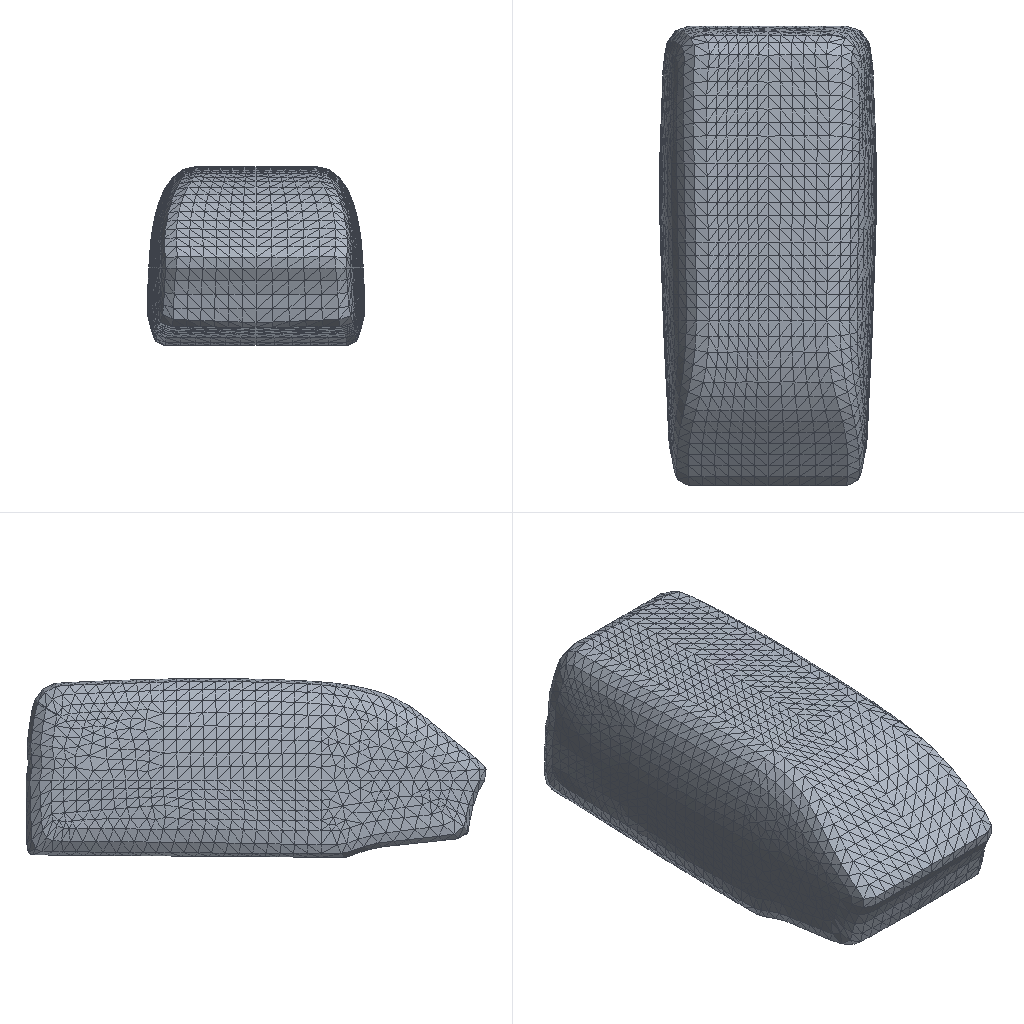Simulation study | abaqus
Set-up summary:
category,name,step,type,value,unit,region
solver,abaqus
solver,version,,,Abaqus/Standard 2020
units,not stated in the deck,,not stated
analysis,deck,,static,static
load_step,Step-1,Step-1,static
load_step,requested,,,1
mesh,nodes,,,7411
mesh,elements,,,37750
element_type,C3D4,,solid,37750
load,load commands in deck,,count,5
bc,support commands in deck,,count,2
material,MATERIAL-1,,in results
check,setup vs results,,match,"per instance, exact: element labels, types and connectivity; labels of the nodes the elements use; coordinates of those nodes at SINGLE_PRECISION in 1 of 1 instance(s)"
Abaqus input file, long lists of numbers shortened:
*Heading
** Job name: Job-3 Model name: Model-3
** Generated by: Abaqus/CAE 2020
*Preprint, echo=NO, model=NO, history=NO, contact=NO
**
** PARTS
**
*Part, name=car3
*Node
      1,   6696.368,        2333.,   520.596
      2,    6753.329,   1345.336,   -47.678
** (7409 more lines like these left out)
*Element, type=C3D4
    1, 2254, 2255, 2256, 2257
    2, 2254, 2256, 2258, 2259
** (37748 more lines like these left out)
*Nset, nset=Set-5, generate
    1,  7411,     1
*Elset, elset=Set-5, generate
     1,  37750,      1
** Section: Section-1
*Solid Section, elset=Set-5, material=Material-1
,
*End Part
**
**
** ASSEMBLY
**
*Assembly, name=Assembly
**
*Instance, name=car3-1, part=car3
*End Instance
**
*Node
      1,   6003.251,   1382.023,  -167.344
*Nset, nset=Set-1, instance=car3-1
    1,    2,    3,    4,    7,    9,   10,   11,   12,   13,   14,   17,   18,   19,   20,   22
   24,   25,   35,   37,   38,   40,   41,   47,   48,   51,   52,   55,   56,   57,   58,   60
** (41 more lines like these left out)
*Elset, elset=Set-1, instance=car3-1
   344,   416,   559,   823,  1168,  1393,  1583,  1620,  2065,  2093,  2105,  2139,  2392,  2495,  2498,  2530
  2554,  2560,  2567,  2572,  2579,  2583,  2603,  2620,  2644,  2647,  2648,  2671,  2673,  2676,  2677,  2683
** (68 more lines like these left out)
*Nset, nset=Set-4
 1,
*Nset, nset=m_Set-2
 1,
*Nset, nset=s_Set-2, instance=car3-1
   29,   30,   42,  283,  284,  285,  286,  287,  288,  289,  290,  291,  292,  293,  294,  295
  296,  297,  298,  299,  300,  301,  302,  303,  304,  382,  383,  384,  385,  386,  387,  388
** (6 more lines like these left out)
*Elset, elset=s_Set-2, instance=car3-1
  2316,  2317,  2608,  2732,  2791,  2832,  2979,  3086,  3128,  3158,  3826,  3863,  3878,  3887,  3889,  4278
  4320,  4345,  4360,  4364,  4367,  4375,  4383,  4407,  4409,  4415,  4429,  4472,  4497,  4509,  4541,  4543
** (12 more lines like these left out)
*Elset, elset=_Surf-1_S2, internal, instance=car3-1
   283,  3506,  3571,  3768,  4714,  5221,  5234,  5363,  5465,  7511, 19785, 23410, 25854
*Elset, elset=_Surf-1_S3, internal, instance=car3-1
   555,   614,  1939,  2150,  2281,  2592,  2668,  2698,  2714,  2740,  2771,  2981,  2997,  3073,  3129,  3131
  3161,  3234,  3238,  3257,  3269,  3308,  3318,  3321,  3339,  3341,  3361,  3368,  3369,  3370,  3378,  3398
** (10 more lines like these left out)
*Elset, elset=_Surf-1_S1, internal, instance=car3-1
  2723,  3423,  3520,  4402,  4690,  5366, 17848, 19788, 30557, 33192
*Elset, elset=_Surf-1_S4, internal, instance=car3-1
  3097,  4419,  4611,  5518,  9574, 15637, 22914, 28537
*Surface, type=ELEMENT, name=Surf-1
_Surf-1_S2, S2
_Surf-1_S3, S3
_Surf-1_S4, S4
_Surf-1_S1, S1
*Elset, elset=_Surf-2_S4, internal, instance=car3-1
  4787,  8357,  8524, 18935, 26301, 30808
*Elset, elset=_Surf-2_S3, internal, instance=car3-1
  2738,  2746,  2905,  4414,  4444,  5828,  5896,  5952,  5967,  5987,  6014,  6016,  6020,  6080,  6189,  6262
  6264,  6312,  6316,  7020,  7053,  7088,  7938,  7969,  7996,  8008,  8022,  8145,  8146,  8200,  8228,  8254
** (10 more lines like these left out)
*Elset, elset=_Surf-2_S1, internal, instance=car3-1
  8427,  8459, 10691, 10758, 10771, 10842, 12517, 33389
*Elset, elset=_Surf-2_S2, internal, instance=car3-1
  6077,  8487,  8533, 10724, 10790, 10829, 10861, 12797, 12913, 12925, 12928
*Surface, type=ELEMENT, name=Surf-2
_Surf-2_S4, S4
_Surf-2_S3, S3
_Surf-2_S2, S2
_Surf-2_S1, S1
*Elset, elset=_Surf-3_S2, internal, instance=car3-1
   565,  4890,  4985,  6532,  6540,  6563,  6624,  6796,  6997,  7125,  7138,  7158,  7167,  7219,  7230,  7243
  7292,  7364,  7399,  7426,  7477,  7495,  7497,  7504,  7505,  7584,  8959,  9052,  9270,  9381,  9425,  9465
** (1 more lines like these left out)
*Elset, elset=_Surf-3_S4, internal, instance=car3-1
  4031,  5815,  6427,  6502,  6551,  6579,  6684,  6856,  6953,  7166,  7227,  9003,  9009,  9098,  9460, 11172
 15746, 17208, 17833, 18163, 19084, 20035, 20091, 20180, 22989, 23093, 28971, 30767
*Elset, elset=_Surf-3_S3, internal, instance=car3-1
   176,   641,  1018,  1963,  2439,  2541,  2555,  2563,  2569,  2587,  2615,  2674,  2755,  2756,  2804,  2848
  2862,  2863,  2879,  3039,  3052,  3084,  3137,  3138,  3142,  3164,  3178,  3206,  3207,  3289,  3299,  3804
** (26 more lines like these left out)
*Elset, elset=_Surf-3_S1, internal, instance=car3-1
  2710,  2801,  6799,  6939,  7116,  7122,  7232,  7315,  7347,  7763,  9398,  9434,  9440,  9618,  9715, 18188
 18454, 18783, 21910
*Surface, type=ELEMENT, name=Surf-3
_Surf-3_S2, S2
_Surf-3_S4, S4
_Surf-3_S3, S3
_Surf-3_S1, S1
*Elset, elset=_Surf-4_S3, internal, instance=car3-1
   172,   199,   264,   338,   383,   385,   506,   507,   552,   702,   742,   814,   913,  1074,  1223,  1323
  1420,  1506,  1787,  1999,  2003,  2026,  2138,  2438,  2645,  2646,  2654,  2798,  2802,  2818,  2821,  2831
** (48 more lines like these left out)
*Elset, elset=_Surf-4_S4, internal, instance=car3-1
   542,   595,   615,  1200,  2898,  6828,  7098,  8867,  9901, 10136, 10216, 10651, 10905, 10916, 10953, 10955
 10991, 11003, 11004, 11982, 12219, 12435, 12469, 13809, 14147, 14288, 14465, 14514, 14516, 14794, 14815, 14817
** (2 more lines like these left out)
*Elset, elset=_Surf-4_S1, internal, instance=car3-1
  2222,  6486, 10188, 10192, 10953, 10955, 10978, 11061, 11134, 12097, 12230, 12427, 13067, 13286, 13291, 13295
 14474, 14534, 14700, 14817, 14841, 14870, 15174, 15372, 15736, 15782, 16801, 17372, 18348, 18819, 21219, 22576
** (1 more lines like these left out)
*Elset, elset=_Surf-4_S2, internal, instance=car3-1
   232,  2380,  2384,  2499,  2759,  7328,  8589,  8633,  8809,  9249, 10320, 10744, 10906, 10922, 10978, 10991
 11038, 12073, 12160, 12183, 12216, 12219, 12399, 12411, 12760, 13072, 13215, 13321, 13323, 13729, 13755, 13798
** (1 more lines like these left out)
*Surface, type=ELEMENT, name=Surf-4
_Surf-4_S3, S3
_Surf-4_S4, S4
_Surf-4_S2, S2
_Surf-4_S1, S1
*Surface, type=NODE, name=s_Set-2_CNS_, internal
s_Set-2, 1.
** Constraint: Constraint-1
*Coupling, constraint name=Constraint-1, ref node=m_Set-2, surface=s_Set-2_CNS_
*Kinematic
*End Assembly
*Amplitude, name=Amp-1, definition=PERIODIC
1,           1256.,              0.,              0.
          1.823,              0.
**
** MATERIALS
**
*Material, name=Material-1
*Density
7890.,
*Elastic
 2.1e+11, 0.3
** ----------------------------------------------------------------
**
** STEP: Step-1
**
*Step, name=Step-1, nlgeom=YES, inc=1000
*Static, stabilize=0.0002, allsdtol=0.05, continue=NO
0.001, 0.1, 1e-06, 0.1
**
** BOUNDARY CONDITIONS
**
** Name: BC-1 Type: 对称/反对称/完全固定
*Boundary
Set-1, ENCASTRE
** Name: BC-2 Type: 速度/角速度
*Boundary, amplitude=Amp-1, type=VELOCITY
Set-4, 1, 1, 1.
**
** LOADS
**
** Name: Load-1   Type: Pressure
*Dsload
Surf-1, P, 0.117
** Name: Load-2   Type: Pressure
*Dsload
Surf-2, P, 0.117
** Name: Load-3   Type: Pressure
*Dsload
Surf-3, P, 0.117
** Name: Load-4   Type: Pressure
*Dsload
Surf-4, P, 0.117
**
** OUTPUT REQUESTS
**
*Restart, write, frequency=0
**
** FIELD OUTPUT: F-Output-1
**
*Output, field
*Node Output
CF, RF, TF, U, V
*Element Output, directions=YES
CTSHR, LE, MISES, NFORC, P, PE, PEEQ, PEMAG, S, SF, SSAVG, TSHR
*Contact Output
CDISP, CSTRESS
**
** HISTORY OUTPUT: H-Output-1
**
*Output, history, variable=PRESELECT
*End Step
Results summary:
result,step,,completed,increments=12 time=0.1/0.1
result,analysis,,,static
result,last_loadstep,,,1
result,primary field,,,U
result,reaction total,,FX,-41613726.498,model units
result,reaction total,,FY,59377.333,model units
result,reaction total,,FZ,157024.551,model units